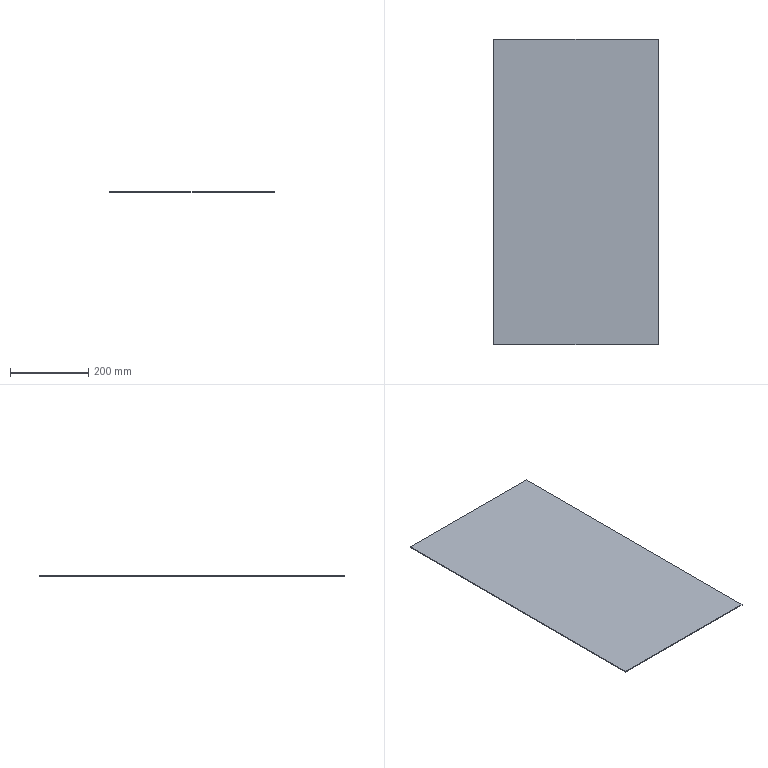Part | STEP file | Acrylic cabinet door | 1 solid | 6 faces | box 418.495 x 778.997 x 2 mm | volume 652013 mm3 | plane 6
STEP:
#1=CARTESIAN_POINT('',(209.248,-389.498,0.));
#2=VERTEX_POINT('',#1);
#3=CARTESIAN_POINT('',(209.248,389.498,0.));
#4=VERTEX_POINT('',#3);
#5=CARTESIAN_POINT('',(209.248,-389.498,0.));
#6=DIRECTION('',(0.,1.,0.));
#7=VECTOR('',#6,1000.);
#8=LINE('',#5,#7);
#9=EDGE_CURVE('',#2,#4,#8,.T.);
#10=ORIENTED_EDGE('',*,*,#9,.T.);
#11=CARTESIAN_POINT('',(209.248,389.498,2.));
#12=VERTEX_POINT('',#11);
#13=CARTESIAN_POINT('',(209.248,389.498,2.));
#14=DIRECTION('',(0.,0.,-1.));
#15=VECTOR('',#14,1000.);
#16=LINE('',#13,#15);
#17=EDGE_CURVE('',#12,#4,#16,.T.);
#18=ORIENTED_EDGE('',*,*,#17,.F.);
#19=CARTESIAN_POINT('',(209.248,-389.498,2.));
#20=VERTEX_POINT('',#19);
#21=CARTESIAN_POINT('',(209.248,-389.498,2.));
#22=DIRECTION('',(0.,1.,0.));
#23=VECTOR('',#22,1000.);
#24=LINE('',#21,#23);
#25=EDGE_CURVE('',#20,#12,#24,.T.);
#26=ORIENTED_EDGE('',*,*,#25,.F.);
#27=CARTESIAN_POINT('',(209.248,-389.498,2.));
#28=DIRECTION('',(0.,0.,-1.));
#29=VECTOR('',#28,1000.);
#30=LINE('',#27,#29);
#31=EDGE_CURVE('',#20,#2,#30,.T.);
#32=ORIENTED_EDGE('',*,*,#31,.T.);
#33=EDGE_LOOP('',(#10,#18,#26,#32));
#34=FACE_OUTER_BOUND('',#33,.T.);
#35=CARTESIAN_POINT('',(209.248,-389.498,2.));
#36=DIRECTION('',(-1.,0.,0.));
#37=DIRECTION('',(0.,0.,1.));
#38=AXIS2_PLACEMENT_3D('',#35,#36,#37);
#39=PLANE('',#38);
#40=ADVANCED_FACE('',(#34),#39,.F.);
#41=CARTESIAN_POINT('',(-209.248,389.498,0.));
#42=VERTEX_POINT('',#41);
#43=CARTESIAN_POINT('',(-209.248,389.498,0.));
#44=DIRECTION('',(-1.,0.,0.));
#45=VECTOR('',#44,1000.);
#46=LINE('',#43,#45);
#47=EDGE_CURVE('',#4,#42,#46,.T.);
#48=ORIENTED_EDGE('',*,*,#47,.T.);
#49=CARTESIAN_POINT('',(-209.248,389.498,2.));
#50=VERTEX_POINT('',#49);
#51=CARTESIAN_POINT('',(-209.248,389.498,2.));
#52=DIRECTION('',(0.,0.,-1.));
#53=VECTOR('',#52,1000.);
#54=LINE('',#51,#53);
#55=EDGE_CURVE('',#50,#42,#54,.T.);
#56=ORIENTED_EDGE('',*,*,#55,.F.);
#57=CARTESIAN_POINT('',(-209.248,389.498,2.));
#58=DIRECTION('',(-1.,0.,0.));
#59=VECTOR('',#58,1000.);
#60=LINE('',#57,#59);
#61=EDGE_CURVE('',#12,#50,#60,.T.);
#62=ORIENTED_EDGE('',*,*,#61,.F.);
#63=ORIENTED_EDGE('',*,*,#17,.T.);
#64=EDGE_LOOP('',(#48,#56,#62,#63));
#65=FACE_OUTER_BOUND('',#64,.T.);
#66=CARTESIAN_POINT('',(-209.248,389.498,2.));
#67=DIRECTION('',(0.,-1.,0.));
#68=DIRECTION('',(0.,0.,-1.));
#69=AXIS2_PLACEMENT_3D('',#66,#67,#68);
#70=PLANE('',#69);
#71=ADVANCED_FACE('',(#65),#70,.F.);
#72=CARTESIAN_POINT('',(-209.248,-389.498,0.));
#73=VERTEX_POINT('',#72);
#74=CARTESIAN_POINT('',(-209.248,-389.498,0.));
#75=DIRECTION('',(0.,-1.,0.));
#76=VECTOR('',#75,1000.);
#77=LINE('',#74,#76);
#78=EDGE_CURVE('',#42,#73,#77,.T.);
#79=ORIENTED_EDGE('',*,*,#78,.T.);
#80=CARTESIAN_POINT('',(-209.248,-389.498,2.));
#81=VERTEX_POINT('',#80);
#82=CARTESIAN_POINT('',(-209.248,-389.498,2.));
#83=DIRECTION('',(0.,0.,-1.));
#84=VECTOR('',#83,1000.);
#85=LINE('',#82,#84);
#86=EDGE_CURVE('',#81,#73,#85,.T.);
#87=ORIENTED_EDGE('',*,*,#86,.F.);
#88=CARTESIAN_POINT('',(-209.248,-389.498,2.));
#89=DIRECTION('',(0.,-1.,0.));
#90=VECTOR('',#89,1000.);
#91=LINE('',#88,#90);
#92=EDGE_CURVE('',#50,#81,#91,.T.);
#93=ORIENTED_EDGE('',*,*,#92,.F.);
#94=ORIENTED_EDGE('',*,*,#55,.T.);
#95=EDGE_LOOP('',(#79,#87,#93,#94));
#96=FACE_OUTER_BOUND('',#95,.T.);
#97=CARTESIAN_POINT('',(-209.248,-389.498,2.));
#98=DIRECTION('',(1.,0.,0.));
#99=DIRECTION('',(0.,0.,-1.));
#100=AXIS2_PLACEMENT_3D('',#97,#98,#99);
#101=PLANE('',#100);
#102=ADVANCED_FACE('',(#96),#101,.F.);
#103=CARTESIAN_POINT('',(-209.248,-389.498,0.));
#104=DIRECTION('',(1.,0.,0.));
#105=VECTOR('',#104,1000.);
#106=LINE('',#103,#105);
#107=EDGE_CURVE('',#73,#2,#106,.T.);
#108=ORIENTED_EDGE('',*,*,#107,.T.);
#109=ORIENTED_EDGE('',*,*,#31,.F.);
#110=CARTESIAN_POINT('',(-209.248,-389.498,2.));
#111=DIRECTION('',(1.,0.,0.));
#112=VECTOR('',#111,1000.);
#113=LINE('',#110,#112);
#114=EDGE_CURVE('',#81,#20,#113,.T.);
#115=ORIENTED_EDGE('',*,*,#114,.F.);
#116=ORIENTED_EDGE('',*,*,#86,.T.);
#117=EDGE_LOOP('',(#108,#109,#115,#116));
#118=FACE_OUTER_BOUND('',#117,.T.);
#119=CARTESIAN_POINT('',(-209.248,-389.498,2.));
#120=DIRECTION('',(0.,1.,0.));
#121=DIRECTION('',(0.,0.,1.));
#122=AXIS2_PLACEMENT_3D('',#119,#120,#121);
#123=PLANE('',#122);
#124=ADVANCED_FACE('',(#118),#123,.F.);
#125=ORIENTED_EDGE('',*,*,#25,.T.);
#126=ORIENTED_EDGE('',*,*,#61,.T.);
#127=ORIENTED_EDGE('',*,*,#92,.T.);
#128=ORIENTED_EDGE('',*,*,#114,.T.);
#129=EDGE_LOOP('',(#125,#126,#127,#128));
#130=FACE_OUTER_BOUND('',#129,.T.);
#131=CARTESIAN_POINT('',(0.,0.,2.));
#132=DIRECTION('',(0.,0.,-1.));
#133=DIRECTION('',(-1.,0.,0.));
#134=AXIS2_PLACEMENT_3D('',#131,#132,#133);
#135=PLANE('',#134);
#136=ADVANCED_FACE('',(#130),#135,.F.);
#137=ORIENTED_EDGE('',*,*,#9,.F.);
#138=ORIENTED_EDGE('',*,*,#107,.F.);
#139=ORIENTED_EDGE('',*,*,#78,.F.);
#140=ORIENTED_EDGE('',*,*,#47,.F.);
#141=EDGE_LOOP('',(#137,#138,#139,#140));
#142=FACE_OUTER_BOUND('',#141,.T.);
#143=CARTESIAN_POINT('',(0.,0.,0.));
#144=DIRECTION('',(0.,0.,-1.));
#145=DIRECTION('',(-1.,0.,0.));
#146=AXIS2_PLACEMENT_3D('',#143,#144,#145);
#147=PLANE('',#146);
#148=ADVANCED_FACE('',(#142),#147,.T.);
#149=CLOSED_SHELL('',(#40,#71,#102,#124,#136,#148));
#150=MANIFOLD_SOLID_BREP('',#149);
#151=CARTESIAN_POINT('',(0.,0.,0.));
#152=DIRECTION('',(0.,0.,1.));
#153=DIRECTION('',(1.,0.,0.));
#154=AXIS2_PLACEMENT_3D('',#151,#152,#153);
#155=(LENGTH_UNIT()NAMED_UNIT(*)SI_UNIT(.MILLI.,.METRE.));
#156=UNCERTAINTY_MEASURE_WITH_UNIT(LENGTH_MEASURE(0.00001),#155,'','');
#157=(NAMED_UNIT(*)PLANE_ANGLE_UNIT()SI_UNIT($,.RADIAN.));
#158=(NAMED_UNIT(*)SI_UNIT($,.STERADIAN.)SOLID_ANGLE_UNIT());
#159=(GEOMETRIC_REPRESENTATION_CONTEXT(3)GLOBAL_UNCERTAINTY_ASSIGNED_CONTEXT((#156))GLOBAL_UNIT_ASSIGNED_CONTEXT((#155,#157,#158))REPRESENTATION_CONTEXT('',''));
#160=ADVANCED_BREP_SHAPE_REPRESENTATION('',(#150,#154),#159);